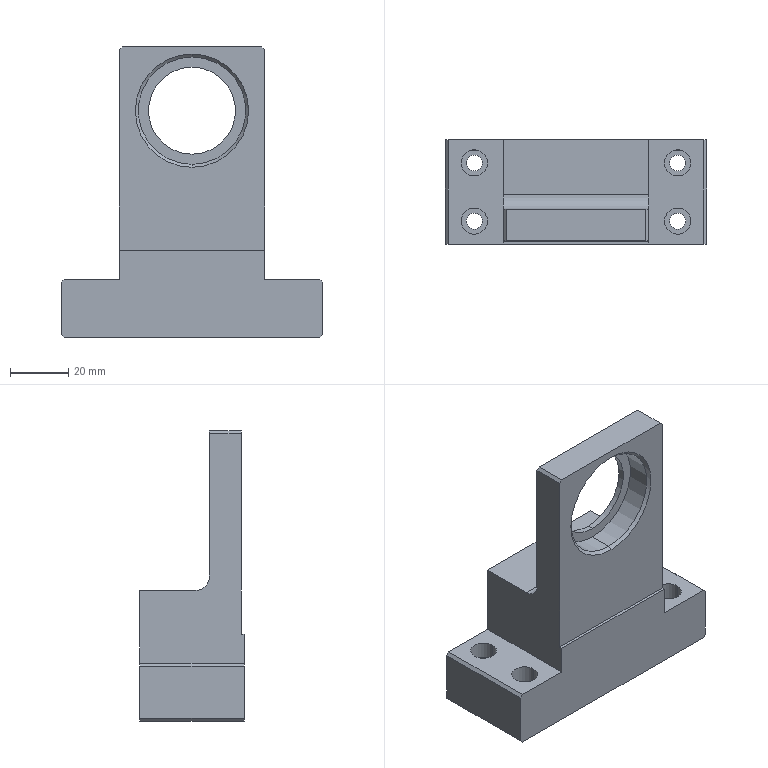Part | NX | features BREP 1 | 1 solid | 64 faces | box 90 x 36 x 100 mm | volume 124790 mm3 | cylinder 29 | plane 25 | cone 10 | commonest cylinder face diameters 4.2 x8 5.5 x8 9 x8 30 x2 37 x2 10 x1